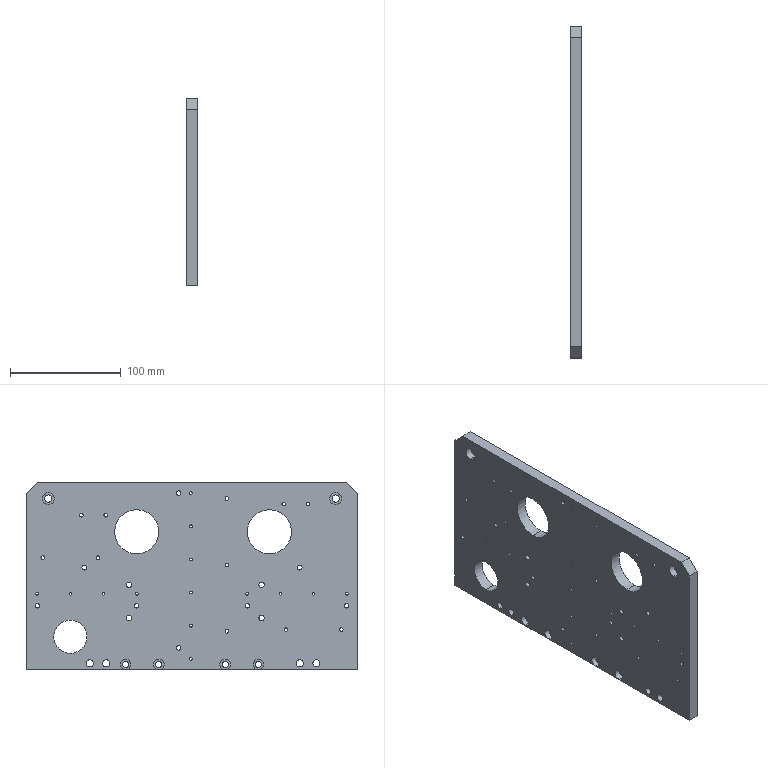Part | SolidWorks | features HoleWzd 17, LPattern 17, Cut 2, ICE 2, Chamfer 1, Extrusion 1, MirrorPattern 1 | 1 solid | 142 faces | box 10 x 300 x 170 mm | volume 468568 mm3 | cylinder 120 | plane 14 | cone 8 | commonest cylinder face diameters 2.5 x36 3.3 x22 4 x12 5 x8 5.5 x8 6.5 x8